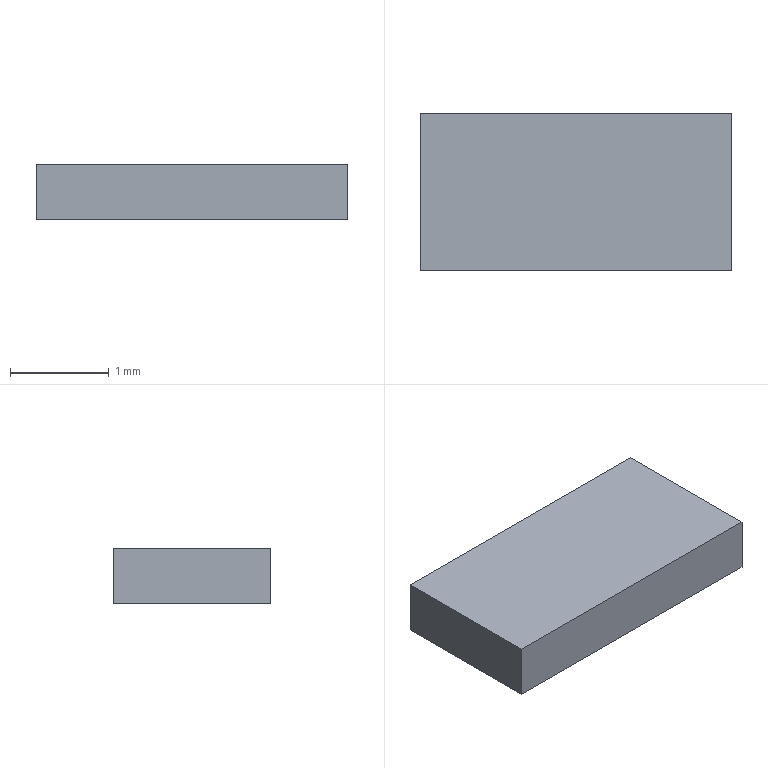Part | STEP file | RJ-USIO-V1_2-220411_98 | 1 solid | 6 faces | box 3.16 x 1.6 x 0.56 mm | volume 2.831 mm3 | plane 6
STEP:
#1=CARTESIAN_POINT('',(0.,0.,0.));
#2=DIRECTION('',(0.,0.,1.));
#3=DIRECTION('',(1.,0.,0.));
#4=AXIS2_PLACEMENT_3D('',#1,#2,#3);
#5=CARTESIAN_POINT('',(80.58,43.2,0.58));
#6=VERTEX_POINT('',#5);
#7=CARTESIAN_POINT('',(80.58,43.2,0.02));
#8=VERTEX_POINT('',#7);
#9=CARTESIAN_POINT('',(80.58,43.2,0.58));
#10=DIRECTION('',(0.,0.,-1.));
#11=VECTOR('',#10,1.);
#12=LINE('',#9,#11);
#13=CARTESIAN_POINT('',(79.,43.2,0.));
#14=DIRECTION('',(-0.000000087,1.,0.));
#15=DIRECTION('',(0.,0.,1.));
#16=AXIS2_PLACEMENT_3D('',#13,#14,#15);
#17=PLANE('',#16);
#18=CARTESIAN_POINT('',(0.58,1.58));
#19=DIRECTION('',(-1.,0.));
#20=VECTOR('',#19,1.);
#21=LINE('',#18,#20);
#22=(GEOMETRIC_REPRESENTATION_CONTEXT(2)PARAMETRIC_REPRESENTATION_CONTEXT()REPRESENTATION_CONTEXT('',''));
#23=DEFINITIONAL_REPRESENTATION('',(#21),#22);
#24=PCURVE('',#17,#23);
#25=CARTESIAN_POINT('',(80.58,44.8,0.58));
#26=DIRECTION('',(1.,0.000000087,0.));
#27=DIRECTION('',(0.,0.,-1.));
#28=AXIS2_PLACEMENT_3D('',#25,#26,#27);
#29=PLANE('',#28);
#30=CARTESIAN_POINT('',(0.,-1.6));
#31=DIRECTION('',(1.,0.));
#32=VECTOR('',#31,1.);
#33=LINE('',#30,#32);
#34=(GEOMETRIC_REPRESENTATION_CONTEXT(2)PARAMETRIC_REPRESENTATION_CONTEXT()REPRESENTATION_CONTEXT('',''));
#35=DEFINITIONAL_REPRESENTATION('',(#33),#34);
#36=PCURVE('',#29,#35);
#37=SURFACE_CURVE('',#12,(#24,#36),.PCURVE_S1.);
#38=EDGE_CURVE('',#6,#8,#37,.T.);
#39=ORIENTED_EDGE('',*,*,#38,.T.);
#40=CARTESIAN_POINT('',(77.42,43.2,0.02));
#41=VERTEX_POINT('',#40);
#42=CARTESIAN_POINT('',(80.58,43.2,0.02));
#43=DIRECTION('',(-1.,-0.000000087,0.));
#44=VECTOR('',#43,1.);
#45=LINE('',#42,#44);
#46=CARTESIAN_POINT('',(0.02,1.58));
#47=DIRECTION('',(0.,-1.));
#48=VECTOR('',#47,1.);
#49=LINE('',#46,#48);
#50=(GEOMETRIC_REPRESENTATION_CONTEXT(2)PARAMETRIC_REPRESENTATION_CONTEXT()REPRESENTATION_CONTEXT('',''));
#51=DEFINITIONAL_REPRESENTATION('',(#49),#50);
#52=PCURVE('',#17,#51);
#53=CARTESIAN_POINT('',(80.58,44.8,0.02));
#54=DIRECTION('',(0.,0.,-1.));
#55=DIRECTION('',(-1.,-0.000000087,0.));
#56=AXIS2_PLACEMENT_3D('',#53,#54,#55);
#57=PLANE('',#56);
#58=CARTESIAN_POINT('',(0.,-1.6));
#59=DIRECTION('',(1.,0.));
#60=VECTOR('',#59,1.);
#61=LINE('',#58,#60);
#62=(GEOMETRIC_REPRESENTATION_CONTEXT(2)PARAMETRIC_REPRESENTATION_CONTEXT()REPRESENTATION_CONTEXT('',''));
#63=DEFINITIONAL_REPRESENTATION('',(#61),#62);
#64=PCURVE('',#57,#63);
#65=SURFACE_CURVE('',#45,(#52,#64),.PCURVE_S1.);
#66=EDGE_CURVE('',#8,#41,#65,.T.);
#67=ORIENTED_EDGE('',*,*,#66,.T.);
#68=CARTESIAN_POINT('',(77.42,43.2,0.58));
#69=VERTEX_POINT('',#68);
#70=CARTESIAN_POINT('',(77.42,43.2,0.02));
#71=DIRECTION('',(0.,0.,1.));
#72=VECTOR('',#71,1.);
#73=LINE('',#70,#72);
#74=CARTESIAN_POINT('',(0.02,-1.58));
#75=DIRECTION('',(1.,0.));
#76=VECTOR('',#75,1.);
#77=LINE('',#74,#76);
#78=(GEOMETRIC_REPRESENTATION_CONTEXT(2)PARAMETRIC_REPRESENTATION_CONTEXT()REPRESENTATION_CONTEXT('',''));
#79=DEFINITIONAL_REPRESENTATION('',(#77),#78);
#80=PCURVE('',#17,#79);
#81=CARTESIAN_POINT('',(77.42,44.8,0.58));
#82=DIRECTION('',(-1.,-0.000000087,0.));
#83=DIRECTION('',(0.,0.,1.));
#84=AXIS2_PLACEMENT_3D('',#81,#82,#83);
#85=PLANE('',#84);
#86=CARTESIAN_POINT('',(-0.56,-1.6));
#87=DIRECTION('',(1.,0.));
#88=VECTOR('',#87,1.);
#89=LINE('',#86,#88);
#90=(GEOMETRIC_REPRESENTATION_CONTEXT(2)PARAMETRIC_REPRESENTATION_CONTEXT()REPRESENTATION_CONTEXT('',''));
#91=DEFINITIONAL_REPRESENTATION('',(#89),#90);
#92=PCURVE('',#85,#91);
#93=SURFACE_CURVE('',#73,(#80,#92),.PCURVE_S1.);
#94=EDGE_CURVE('',#41,#69,#93,.T.);
#95=ORIENTED_EDGE('',*,*,#94,.T.);
#96=CARTESIAN_POINT('',(77.42,43.2,0.58));
#97=DIRECTION('',(1.,0.000000087,0.));
#98=VECTOR('',#97,1.);
#99=LINE('',#96,#98);
#100=CARTESIAN_POINT('',(0.58,-1.58));
#101=DIRECTION('',(0.,1.));
#102=VECTOR('',#101,1.);
#103=LINE('',#100,#102);
#104=(GEOMETRIC_REPRESENTATION_CONTEXT(2)PARAMETRIC_REPRESENTATION_CONTEXT()REPRESENTATION_CONTEXT('',''));
#105=DEFINITIONAL_REPRESENTATION('',(#103),#104);
#106=PCURVE('',#17,#105);
#107=CARTESIAN_POINT('',(80.58,44.8,0.58));
#108=DIRECTION('',(0.,0.,1.));
#109=DIRECTION('',(1.,0.000000087,0.));
#110=AXIS2_PLACEMENT_3D('',#107,#108,#109);
#111=PLANE('',#110);
#112=CARTESIAN_POINT('',(-3.16,-1.6));
#113=DIRECTION('',(1.,0.));
#114=VECTOR('',#113,1.);
#115=LINE('',#112,#114);
#116=(GEOMETRIC_REPRESENTATION_CONTEXT(2)PARAMETRIC_REPRESENTATION_CONTEXT()REPRESENTATION_CONTEXT('',''));
#117=DEFINITIONAL_REPRESENTATION('',(#115),#116);
#118=PCURVE('',#111,#117);
#119=SURFACE_CURVE('',#99,(#106,#118),.PCURVE_S1.);
#120=EDGE_CURVE('',#69,#6,#119,.T.);
#121=ORIENTED_EDGE('',*,*,#120,.T.);
#122=EDGE_LOOP('',(#39,#67,#95,#121));
#123=FACE_BOUND('',#122,.F.);
#124=ADVANCED_FACE('',(#123),#17,.F.);
#125=CARTESIAN_POINT('',(80.58,44.8,0.58));
#126=VERTEX_POINT('',#125);
#127=CARTESIAN_POINT('',(80.58,43.2,0.58));
#128=DIRECTION('',(-0.000000087,1.,0.));
#129=VECTOR('',#128,1.);
#130=LINE('',#127,#129);
#131=CARTESIAN_POINT('',(0.,-1.6));
#132=DIRECTION('',(0.,1.));
#133=VECTOR('',#132,1.);
#134=LINE('',#131,#133);
#135=(GEOMETRIC_REPRESENTATION_CONTEXT(2)PARAMETRIC_REPRESENTATION_CONTEXT()REPRESENTATION_CONTEXT('',''));
#136=DEFINITIONAL_REPRESENTATION('',(#134),#135);
#137=PCURVE('',#29,#136);
#138=CARTESIAN_POINT('',(0.,-1.6));
#139=DIRECTION('',(0.,1.));
#140=VECTOR('',#139,1.);
#141=LINE('',#138,#140);
#142=(GEOMETRIC_REPRESENTATION_CONTEXT(2)PARAMETRIC_REPRESENTATION_CONTEXT()REPRESENTATION_CONTEXT('',''));
#143=DEFINITIONAL_REPRESENTATION('',(#141),#142);
#144=PCURVE('',#111,#143);
#145=SURFACE_CURVE('',#130,(#137,#144),.PCURVE_S1.);
#146=EDGE_CURVE('',#6,#126,#145,.T.);
#147=ORIENTED_EDGE('',*,*,#146,.T.);
#148=CARTESIAN_POINT('',(80.58,44.8,0.02));
#149=VERTEX_POINT('',#148);
#150=CARTESIAN_POINT('',(80.58,44.8,0.58));
#151=DIRECTION('',(0.,0.,-1.));
#152=VECTOR('',#151,1.);
#153=LINE('',#150,#152);
#154=CARTESIAN_POINT('',(0.,0.));
#155=DIRECTION('',(1.,0.));
#156=VECTOR('',#155,1.);
#157=LINE('',#154,#156);
#158=(GEOMETRIC_REPRESENTATION_CONTEXT(2)PARAMETRIC_REPRESENTATION_CONTEXT()REPRESENTATION_CONTEXT('',''));
#159=DEFINITIONAL_REPRESENTATION('',(#157),#158);
#160=PCURVE('',#29,#159);
#161=CARTESIAN_POINT('',(79.,44.8,0.));
#162=DIRECTION('',(-0.000000087,1.,0.));
#163=DIRECTION('',(0.,0.,1.));
#164=AXIS2_PLACEMENT_3D('',#161,#162,#163);
#165=PLANE('',#164);
#166=CARTESIAN_POINT('',(0.58,1.58));
#167=DIRECTION('',(-1.,0.));
#168=VECTOR('',#167,1.);
#169=LINE('',#166,#168);
#170=(GEOMETRIC_REPRESENTATION_CONTEXT(2)PARAMETRIC_REPRESENTATION_CONTEXT()REPRESENTATION_CONTEXT('',''));
#171=DEFINITIONAL_REPRESENTATION('',(#169),#170);
#172=PCURVE('',#165,#171);
#173=SURFACE_CURVE('',#153,(#160,#172),.PCURVE_S1.);
#174=EDGE_CURVE('',#126,#149,#173,.T.);
#175=ORIENTED_EDGE('',*,*,#174,.T.);
#176=CARTESIAN_POINT('',(80.58,43.2,0.02));
#177=DIRECTION('',(-0.000000087,1.,0.));
#178=VECTOR('',#177,1.);
#179=LINE('',#176,#178);
#180=CARTESIAN_POINT('',(0.56,-1.6));
#181=DIRECTION('',(0.,1.));
#182=VECTOR('',#181,1.);
#183=LINE('',#180,#182);
#184=(GEOMETRIC_REPRESENTATION_CONTEXT(2)PARAMETRIC_REPRESENTATION_CONTEXT()REPRESENTATION_CONTEXT('',''));
#185=DEFINITIONAL_REPRESENTATION('',(#183),#184);
#186=PCURVE('',#29,#185);
#187=CARTESIAN_POINT('',(0.,-1.6));
#188=DIRECTION('',(0.,1.));
#189=VECTOR('',#188,1.);
#190=LINE('',#187,#189);
#191=(GEOMETRIC_REPRESENTATION_CONTEXT(2)PARAMETRIC_REPRESENTATION_CONTEXT()REPRESENTATION_CONTEXT('',''));
#192=DEFINITIONAL_REPRESENTATION('',(#190),#191);
#193=PCURVE('',#57,#192);
#194=SURFACE_CURVE('',#179,(#186,#193),.PCURVE_S1.);
#195=EDGE_CURVE('',#8,#149,#194,.T.);
#196=ORIENTED_EDGE('',*,*,#195,.F.);
#197=ORIENTED_EDGE('',*,*,#38,.F.);
#198=EDGE_LOOP('',(#147,#175,#196,#197));
#199=FACE_BOUND('',#198,.F.);
#200=ADVANCED_FACE('',(#199),#29,.T.);
#201=CARTESIAN_POINT('',(77.42,44.8,0.58));
#202=VERTEX_POINT('',#201);
#203=CARTESIAN_POINT('',(77.42,43.2,0.58));
#204=DIRECTION('',(-0.000000087,1.,0.));
#205=VECTOR('',#204,1.);
#206=LINE('',#203,#205);
#207=CARTESIAN_POINT('',(-3.16,-1.6));
#208=DIRECTION('',(0.,1.));
#209=VECTOR('',#208,1.);
#210=LINE('',#207,#209);
#211=(GEOMETRIC_REPRESENTATION_CONTEXT(2)PARAMETRIC_REPRESENTATION_CONTEXT()REPRESENTATION_CONTEXT('',''));
#212=DEFINITIONAL_REPRESENTATION('',(#210),#211);
#213=PCURVE('',#111,#212);
#214=CARTESIAN_POINT('',(0.,-1.6));
#215=DIRECTION('',(0.,1.));
#216=VECTOR('',#215,1.);
#217=LINE('',#214,#216);
#218=(GEOMETRIC_REPRESENTATION_CONTEXT(2)PARAMETRIC_REPRESENTATION_CONTEXT()REPRESENTATION_CONTEXT('',''));
#219=DEFINITIONAL_REPRESENTATION('',(#217),#218);
#220=PCURVE('',#85,#219);
#221=SURFACE_CURVE('',#206,(#213,#220),.PCURVE_S1.);
#222=EDGE_CURVE('',#69,#202,#221,.T.);
#223=ORIENTED_EDGE('',*,*,#222,.T.);
#224=CARTESIAN_POINT('',(77.42,44.8,0.58));
#225=DIRECTION('',(1.,0.000000087,0.));
#226=VECTOR('',#225,1.);
#227=LINE('',#224,#226);
#228=CARTESIAN_POINT('',(-3.16,0.));
#229=DIRECTION('',(1.,0.));
#230=VECTOR('',#229,1.);
#231=LINE('',#228,#230);
#232=(GEOMETRIC_REPRESENTATION_CONTEXT(2)PARAMETRIC_REPRESENTATION_CONTEXT()REPRESENTATION_CONTEXT('',''));
#233=DEFINITIONAL_REPRESENTATION('',(#231),#232);
#234=PCURVE('',#111,#233);
#235=CARTESIAN_POINT('',(0.58,-1.58));
#236=DIRECTION('',(0.,1.));
#237=VECTOR('',#236,1.);
#238=LINE('',#235,#237);
#239=(GEOMETRIC_REPRESENTATION_CONTEXT(2)PARAMETRIC_REPRESENTATION_CONTEXT()REPRESENTATION_CONTEXT('',''));
#240=DEFINITIONAL_REPRESENTATION('',(#238),#239);
#241=PCURVE('',#165,#240);
#242=SURFACE_CURVE('',#227,(#234,#241),.PCURVE_S1.);
#243=EDGE_CURVE('',#202,#126,#242,.T.);
#244=ORIENTED_EDGE('',*,*,#243,.T.);
#245=ORIENTED_EDGE('',*,*,#146,.F.);
#246=ORIENTED_EDGE('',*,*,#120,.F.);
#247=EDGE_LOOP('',(#223,#244,#245,#246));
#248=FACE_BOUND('',#247,.F.);
#249=ADVANCED_FACE('',(#248),#111,.T.);
#250=CARTESIAN_POINT('',(77.42,44.8,0.02));
#251=VERTEX_POINT('',#250);
#252=CARTESIAN_POINT('',(77.42,43.2,0.02));
#253=DIRECTION('',(-0.000000087,1.,0.));
#254=VECTOR('',#253,1.);
#255=LINE('',#252,#254);
#256=CARTESIAN_POINT('',(-0.56,-1.6));
#257=DIRECTION('',(0.,1.));
#258=VECTOR('',#257,1.);
#259=LINE('',#256,#258);
#260=(GEOMETRIC_REPRESENTATION_CONTEXT(2)PARAMETRIC_REPRESENTATION_CONTEXT()REPRESENTATION_CONTEXT('',''));
#261=DEFINITIONAL_REPRESENTATION('',(#259),#260);
#262=PCURVE('',#85,#261);
#263=CARTESIAN_POINT('',(3.16,-1.6));
#264=DIRECTION('',(0.,1.));
#265=VECTOR('',#264,1.);
#266=LINE('',#263,#265);
#267=(GEOMETRIC_REPRESENTATION_CONTEXT(2)PARAMETRIC_REPRESENTATION_CONTEXT()REPRESENTATION_CONTEXT('',''));
#268=DEFINITIONAL_REPRESENTATION('',(#266),#267);
#269=PCURVE('',#57,#268);
#270=SURFACE_CURVE('',#255,(#262,#269),.PCURVE_S1.);
#271=EDGE_CURVE('',#41,#251,#270,.T.);
#272=ORIENTED_EDGE('',*,*,#271,.T.);
#273=CARTESIAN_POINT('',(77.42,44.8,0.02));
#274=DIRECTION('',(0.,0.,1.));
#275=VECTOR('',#274,1.);
#276=LINE('',#273,#275);
#277=CARTESIAN_POINT('',(-0.56,0.));
#278=DIRECTION('',(1.,0.));
#279=VECTOR('',#278,1.);
#280=LINE('',#277,#279);
#281=(GEOMETRIC_REPRESENTATION_CONTEXT(2)PARAMETRIC_REPRESENTATION_CONTEXT()REPRESENTATION_CONTEXT('',''));
#282=DEFINITIONAL_REPRESENTATION('',(#280),#281);
#283=PCURVE('',#85,#282);
#284=CARTESIAN_POINT('',(0.02,-1.58));
#285=DIRECTION('',(1.,0.));
#286=VECTOR('',#285,1.);
#287=LINE('',#284,#286);
#288=(GEOMETRIC_REPRESENTATION_CONTEXT(2)PARAMETRIC_REPRESENTATION_CONTEXT()REPRESENTATION_CONTEXT('',''));
#289=DEFINITIONAL_REPRESENTATION('',(#287),#288);
#290=PCURVE('',#165,#289);
#291=SURFACE_CURVE('',#276,(#283,#290),.PCURVE_S1.);
#292=EDGE_CURVE('',#251,#202,#291,.T.);
#293=ORIENTED_EDGE('',*,*,#292,.T.);
#294=ORIENTED_EDGE('',*,*,#222,.F.);
#295=ORIENTED_EDGE('',*,*,#94,.F.);
#296=EDGE_LOOP('',(#272,#293,#294,#295));
#297=FACE_BOUND('',#296,.F.);
#298=ADVANCED_FACE('',(#297),#85,.T.);
#299=ORIENTED_EDGE('',*,*,#195,.T.);
#300=CARTESIAN_POINT('',(80.58,44.8,0.02));
#301=DIRECTION('',(-1.,-0.000000087,0.));
#302=VECTOR('',#301,1.);
#303=LINE('',#300,#302);
#304=CARTESIAN_POINT('',(0.,0.));
#305=DIRECTION('',(1.,0.));
#306=VECTOR('',#305,1.);
#307=LINE('',#304,#306);
#308=(GEOMETRIC_REPRESENTATION_CONTEXT(2)PARAMETRIC_REPRESENTATION_CONTEXT()REPRESENTATION_CONTEXT('',''));
#309=DEFINITIONAL_REPRESENTATION('',(#307),#308);
#310=PCURVE('',#57,#309);
#311=CARTESIAN_POINT('',(0.02,1.58));
#312=DIRECTION('',(0.,-1.));
#313=VECTOR('',#312,1.);
#314=LINE('',#311,#313);
#315=(GEOMETRIC_REPRESENTATION_CONTEXT(2)PARAMETRIC_REPRESENTATION_CONTEXT()REPRESENTATION_CONTEXT('',''));
#316=DEFINITIONAL_REPRESENTATION('',(#314),#315);
#317=PCURVE('',#165,#316);
#318=SURFACE_CURVE('',#303,(#310,#317),.PCURVE_S1.);
#319=EDGE_CURVE('',#149,#251,#318,.T.);
#320=ORIENTED_EDGE('',*,*,#319,.T.);
#321=ORIENTED_EDGE('',*,*,#271,.F.);
#322=ORIENTED_EDGE('',*,*,#66,.F.);
#323=EDGE_LOOP('',(#299,#320,#321,#322));
#324=FACE_BOUND('',#323,.F.);
#325=ADVANCED_FACE('',(#324),#57,.T.);
#326=ORIENTED_EDGE('',*,*,#174,.F.);
#327=ORIENTED_EDGE('',*,*,#243,.F.);
#328=ORIENTED_EDGE('',*,*,#292,.F.);
#329=ORIENTED_EDGE('',*,*,#319,.F.);
#330=EDGE_LOOP('',(#326,#327,#328,#329));
#331=FACE_BOUND('',#330,.F.);
#332=ADVANCED_FACE('',(#331),#165,.T.);
#333=CLOSED_SHELL('',(#124,#200,#249,#298,#325,#332));
#334=MANIFOLD_SOLID_BREP('',#333);
#335=(LENGTH_UNIT()NAMED_UNIT(*)SI_UNIT(.MILLI.,.METRE.));
#336=UNCERTAINTY_MEASURE_WITH_UNIT(LENGTH_MEASURE(0.0000001),#335,'','');
#337=(NAMED_UNIT(*)PLANE_ANGLE_UNIT()SI_UNIT($,.RADIAN.));
#338=(NAMED_UNIT(*)SI_UNIT($,.STERADIAN.)SOLID_ANGLE_UNIT());
#339=(GEOMETRIC_REPRESENTATION_CONTEXT(3)GLOBAL_UNCERTAINTY_ASSIGNED_CONTEXT((#336))GLOBAL_UNIT_ASSIGNED_CONTEXT((#335,#337,#338))REPRESENTATION_CONTEXT('',''));
#340=ADVANCED_BREP_SHAPE_REPRESENTATION('',(#4,#334),#339);